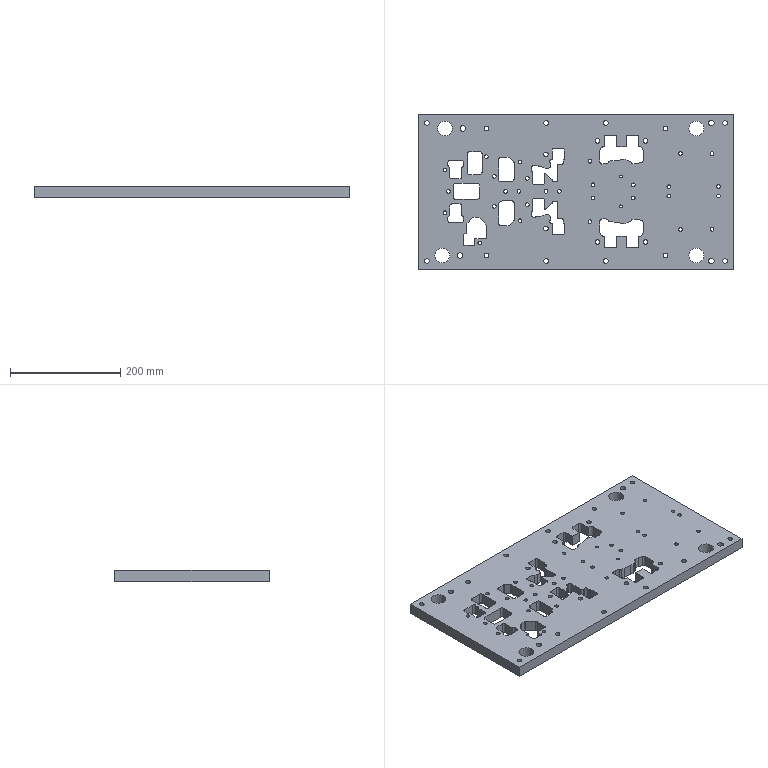Part | NX | features PPS-1 2 | 1 solid | 333 faces | box 570 x 280 x 20 mm | volume 2738315 mm3 | cylinder 146 | plane 108 | spline 46 | cone 33 | commonest cylinder face diameters 7 x32 9 x18 10 x18 6.805 x16 8.5 x16 6.8 x12